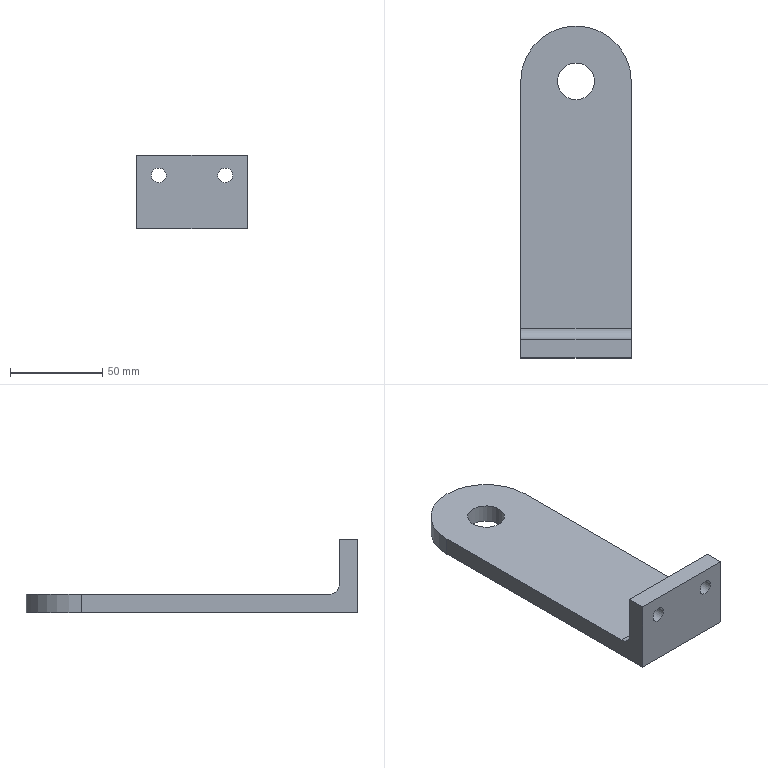Part | STEP file | tieqianzhizhu | 1 solid | 12 faces | box 60 x 180 x 40 mm | volume 118454 mm3 | plane 7 | cylinder 5 | commonest cylinder face diameters 8 x2 12 x1 20 x1 60 x1
STEP:
#1=CARTESIAN_POINT('',(0.,0.,0.));
#2=DIRECTION('',(0.,0.,1.));
#3=DIRECTION('',(1.,0.,0.));
#4=AXIS2_PLACEMENT_3D('',#1,#2,#3);
#5=CARTESIAN_POINT('',(-30.,0.,10.));
#6=VERTEX_POINT('',#5);
#7=CARTESIAN_POINT('',(-30.,-134.,10.));
#8=VERTEX_POINT('',#7);
#9=CARTESIAN_POINT('',(-30.,0.,10.));
#10=DIRECTION('',(0.,-1.,0.));
#11=VECTOR('',#10,1.);
#12=LINE('',#9,#11);
#13=CARTESIAN_POINT('',(0.,0.,10.));
#14=DIRECTION('',(0.,0.,1.));
#15=DIRECTION('',(1.,0.,0.));
#16=AXIS2_PLACEMENT_3D('',#13,#14,#15);
#17=PLANE('',#16);
#18=CARTESIAN_POINT('',(-30.,0.));
#19=DIRECTION('',(0.,-1.));
#20=VECTOR('',#19,1.);
#21=LINE('',#18,#20);
#22=(GEOMETRIC_REPRESENTATION_CONTEXT(2)PARAMETRIC_REPRESENTATION_CONTEXT()REPRESENTATION_CONTEXT('',''));
#23=DEFINITIONAL_REPRESENTATION('',(#21),#22);
#24=PCURVE('',#17,#23);
#25=CARTESIAN_POINT('',(-30.,0.,10.));
#26=DIRECTION('',(1.,0.,0.));
#27=DIRECTION('',(0.,1.,0.));
#28=AXIS2_PLACEMENT_3D('',#25,#26,#27);
#29=PLANE('',#28);
#30=CARTESIAN_POINT('',(0.,0.));
#31=DIRECTION('',(-1.,0.));
#32=VECTOR('',#31,1.);
#33=LINE('',#30,#32);
#34=(GEOMETRIC_REPRESENTATION_CONTEXT(2)PARAMETRIC_REPRESENTATION_CONTEXT()REPRESENTATION_CONTEXT('',''));
#35=DEFINITIONAL_REPRESENTATION('',(#33),#34);
#36=PCURVE('',#29,#35);
#37=SURFACE_CURVE('',#12,(#24,#36),.PCURVE_S1.);
#38=EDGE_CURVE('',#6,#8,#37,.T.);
#39=ORIENTED_EDGE('',*,*,#38,.T.);
#40=CARTESIAN_POINT('',(30.,-134.,10.));
#41=VERTEX_POINT('',#40);
#42=CARTESIAN_POINT('',(0.,-134.,10.));
#43=DIRECTION('',(1.,0.,0.));
#44=VECTOR('',#43,1.);
#45=LINE('',#42,#44);
#46=CARTESIAN_POINT('',(0.,-134.));
#47=DIRECTION('',(1.,0.));
#48=VECTOR('',#47,1.);
#49=LINE('',#46,#48);
#50=(GEOMETRIC_REPRESENTATION_CONTEXT(2)PARAMETRIC_REPRESENTATION_CONTEXT()REPRESENTATION_CONTEXT('',''));
#51=DEFINITIONAL_REPRESENTATION('',(#49),#50);
#52=PCURVE('',#17,#51);
#53=CARTESIAN_POINT('',(-30.,-134.,16.));
#54=DIRECTION('',(-1.,0.,0.));
#55=DIRECTION('',(0.,0.,1.));
#56=AXIS2_PLACEMENT_3D('',#53,#54,#55);
#57=CYLINDRICAL_SURFACE('',#56,6.);
#58=CARTESIAN_POINT('',(3.142,-30.));
#59=DIRECTION('',(0.,-1.));
#60=VECTOR('',#59,1.);
#61=LINE('',#58,#60);
#62=(GEOMETRIC_REPRESENTATION_CONTEXT(2)PARAMETRIC_REPRESENTATION_CONTEXT()REPRESENTATION_CONTEXT('',''));
#63=DEFINITIONAL_REPRESENTATION('',(#61),#62);
#64=PCURVE('',#57,#63);
#65=SURFACE_CURVE('',#45,(#52,#64),.PCURVE_S1.);
#66=EDGE_CURVE('',#8,#41,#65,.T.);
#67=ORIENTED_EDGE('',*,*,#66,.T.);
#68=CARTESIAN_POINT('',(30.,0.,10.));
#69=VERTEX_POINT('',#68);
#70=CARTESIAN_POINT('',(30.,0.,10.));
#71=DIRECTION('',(0.,1.,0.));
#72=VECTOR('',#71,1.);
#73=LINE('',#70,#72);
#74=CARTESIAN_POINT('',(30.,0.));
#75=DIRECTION('',(0.,1.));
#76=VECTOR('',#75,1.);
#77=LINE('',#74,#76);
#78=(GEOMETRIC_REPRESENTATION_CONTEXT(2)PARAMETRIC_REPRESENTATION_CONTEXT()REPRESENTATION_CONTEXT('',''));
#79=DEFINITIONAL_REPRESENTATION('',(#77),#78);
#80=PCURVE('',#17,#79);
#81=CARTESIAN_POINT('',(30.,0.,10.));
#82=DIRECTION('',(-1.,0.,0.));
#83=DIRECTION('',(0.,-1.,0.));
#84=AXIS2_PLACEMENT_3D('',#81,#82,#83);
#85=PLANE('',#84);
#86=CARTESIAN_POINT('',(0.,0.));
#87=DIRECTION('',(-1.,0.));
#88=VECTOR('',#87,1.);
#89=LINE('',#86,#88);
#90=(GEOMETRIC_REPRESENTATION_CONTEXT(2)PARAMETRIC_REPRESENTATION_CONTEXT()REPRESENTATION_CONTEXT('',''));
#91=DEFINITIONAL_REPRESENTATION('',(#89),#90);
#92=PCURVE('',#85,#91);
#93=SURFACE_CURVE('',#73,(#80,#92),.PCURVE_S1.);
#94=EDGE_CURVE('',#41,#69,#93,.T.);
#95=ORIENTED_EDGE('',*,*,#94,.T.);
#96=CARTESIAN_POINT('',(0.,0.,10.));
#97=DIRECTION('',(0.,0.,1.));
#98=DIRECTION('',(1.,0.,0.));
#99=AXIS2_PLACEMENT_3D('',#96,#97,#98);
#100=CIRCLE('',#99,30.);
#101=CARTESIAN_POINT('',(0.,0.));
#102=DIRECTION('',(1.,0.));
#103=AXIS2_PLACEMENT_2D('',#101,#102);
#104=CIRCLE('',#103,30.);
#105=(GEOMETRIC_REPRESENTATION_CONTEXT(2)PARAMETRIC_REPRESENTATION_CONTEXT()REPRESENTATION_CONTEXT('',''));
#106=DEFINITIONAL_REPRESENTATION('',(#104),#105);
#107=PCURVE('',#17,#106);
#108=CARTESIAN_POINT('',(0.,0.,10.));
#109=DIRECTION('',(0.,0.,-1.));
#110=DIRECTION('',(-1.,0.,0.));
#111=AXIS2_PLACEMENT_3D('',#108,#109,#110);
#112=CYLINDRICAL_SURFACE('',#111,30.);
#113=CARTESIAN_POINT('',(3.142,0.));
#114=DIRECTION('',(-1.,0.));
#115=VECTOR('',#114,1.);
#116=LINE('',#113,#115);
#117=(GEOMETRIC_REPRESENTATION_CONTEXT(2)PARAMETRIC_REPRESENTATION_CONTEXT()REPRESENTATION_CONTEXT('',''));
#118=DEFINITIONAL_REPRESENTATION('',(#116),#117);
#119=PCURVE('',#112,#118);
#120=SURFACE_CURVE('',#100,(#107,#119),.PCURVE_S1.);
#121=EDGE_CURVE('',#69,#6,#120,.T.);
#122=ORIENTED_EDGE('',*,*,#121,.T.);
#123=EDGE_LOOP('',(#39,#67,#95,#122));
#124=FACE_BOUND('',#123,.T.);
#125=CARTESIAN_POINT('',(10.,0.,10.));
#126=VERTEX_POINT('',#125);
#127=CARTESIAN_POINT('',(0.,0.,10.));
#128=DIRECTION('',(0.,0.,1.));
#129=DIRECTION('',(1.,0.,0.));
#130=AXIS2_PLACEMENT_3D('',#127,#128,#129);
#131=CIRCLE('',#130,10.);
#132=CARTESIAN_POINT('',(0.,0.));
#133=DIRECTION('',(1.,0.));
#134=AXIS2_PLACEMENT_2D('',#132,#133);
#135=CIRCLE('',#134,10.);
#136=(GEOMETRIC_REPRESENTATION_CONTEXT(2)PARAMETRIC_REPRESENTATION_CONTEXT()REPRESENTATION_CONTEXT('',''));
#137=DEFINITIONAL_REPRESENTATION('',(#135),#136);
#138=PCURVE('',#17,#137);
#139=CARTESIAN_POINT('',(0.,0.,10.));
#140=DIRECTION('',(0.,0.,-1.));
#141=DIRECTION('',(-1.,0.,0.));
#142=AXIS2_PLACEMENT_3D('',#139,#140,#141);
#143=CYLINDRICAL_SURFACE('',#142,10.);
#144=CARTESIAN_POINT('',(9.425,0.));
#145=DIRECTION('',(-1.,0.));
#146=VECTOR('',#145,1.);
#147=LINE('',#144,#146);
#148=(GEOMETRIC_REPRESENTATION_CONTEXT(2)PARAMETRIC_REPRESENTATION_CONTEXT()REPRESENTATION_CONTEXT('',''));
#149=DEFINITIONAL_REPRESENTATION('',(#147),#148);
#150=PCURVE('',#143,#149);
#151=SURFACE_CURVE('',#131,(#138,#150),.PCURVE_S1.);
#152=EDGE_CURVE('',#126,#126,#151,.T.);
#153=ORIENTED_EDGE('',*,*,#152,.F.);
#154=EDGE_LOOP('',(#153));
#155=FACE_BOUND('',#154,.T.);
#156=ADVANCED_FACE('',(#124,#155),#17,.T.);
#157=CARTESIAN_POINT('',(30.,0.,0.));
#158=VERTEX_POINT('',#157);
#159=CARTESIAN_POINT('',(-30.,0.,0.));
#160=VERTEX_POINT('',#159);
#161=CARTESIAN_POINT('',(0.,0.,0.));
#162=DIRECTION('',(0.,0.,1.));
#163=DIRECTION('',(1.,0.,0.));
#164=AXIS2_PLACEMENT_3D('',#161,#162,#163);
#165=CIRCLE('',#164,30.);
#166=CARTESIAN_POINT('',(0.,0.,0.));
#167=DIRECTION('',(0.,0.,1.));
#168=DIRECTION('',(1.,0.,0.));
#169=AXIS2_PLACEMENT_3D('',#166,#167,#168);
#170=PLANE('',#169);
#171=CARTESIAN_POINT('',(0.,0.));
#172=DIRECTION('',(1.,0.));
#173=AXIS2_PLACEMENT_2D('',#171,#172);
#174=CIRCLE('',#173,30.);
#175=(GEOMETRIC_REPRESENTATION_CONTEXT(2)PARAMETRIC_REPRESENTATION_CONTEXT()REPRESENTATION_CONTEXT('',''));
#176=DEFINITIONAL_REPRESENTATION('',(#174),#175);
#177=PCURVE('',#170,#176);
#178=CARTESIAN_POINT('',(3.142,10.));
#179=DIRECTION('',(-1.,0.));
#180=VECTOR('',#179,1.);
#181=LINE('',#178,#180);
#182=(GEOMETRIC_REPRESENTATION_CONTEXT(2)PARAMETRIC_REPRESENTATION_CONTEXT()REPRESENTATION_CONTEXT('',''));
#183=DEFINITIONAL_REPRESENTATION('',(#181),#182);
#184=PCURVE('',#112,#183);
#185=SURFACE_CURVE('',#165,(#177,#184),.PCURVE_S1.);
#186=EDGE_CURVE('',#158,#160,#185,.T.);
#187=ORIENTED_EDGE('',*,*,#186,.F.);
#188=CARTESIAN_POINT('',(30.,-150.,0.));
#189=VERTEX_POINT('',#188);
#190=CARTESIAN_POINT('',(30.,0.,0.));
#191=DIRECTION('',(0.,1.,0.));
#192=VECTOR('',#191,1.);
#193=LINE('',#190,#192);
#194=CARTESIAN_POINT('',(30.,0.));
#195=DIRECTION('',(0.,1.));
#196=VECTOR('',#195,1.);
#197=LINE('',#194,#196);
#198=(GEOMETRIC_REPRESENTATION_CONTEXT(2)PARAMETRIC_REPRESENTATION_CONTEXT()REPRESENTATION_CONTEXT('',''));
#199=DEFINITIONAL_REPRESENTATION('',(#197),#198);
#200=PCURVE('',#170,#199);
#201=CARTESIAN_POINT('',(0.,-10.));
#202=DIRECTION('',(-1.,0.));
#203=VECTOR('',#202,1.);
#204=LINE('',#201,#203);
#205=(GEOMETRIC_REPRESENTATION_CONTEXT(2)PARAMETRIC_REPRESENTATION_CONTEXT()REPRESENTATION_CONTEXT('',''));
#206=DEFINITIONAL_REPRESENTATION('',(#204),#205);
#207=PCURVE('',#85,#206);
#208=SURFACE_CURVE('',#193,(#200,#207),.PCURVE_S1.);
#209=EDGE_CURVE('',#189,#158,#208,.T.);
#210=ORIENTED_EDGE('',*,*,#209,.F.);
#211=CARTESIAN_POINT('',(-30.,-150.,0.));
#212=VERTEX_POINT('',#211);
#213=CARTESIAN_POINT('',(30.,-150.,0.));
#214=DIRECTION('',(1.,0.,0.));
#215=VECTOR('',#214,1.);
#216=LINE('',#213,#215);
#217=CARTESIAN_POINT('',(30.,-150.));
#218=DIRECTION('',(1.,0.));
#219=VECTOR('',#218,1.);
#220=LINE('',#217,#219);
#221=(GEOMETRIC_REPRESENTATION_CONTEXT(2)PARAMETRIC_REPRESENTATION_CONTEXT()REPRESENTATION_CONTEXT('',''));
#222=DEFINITIONAL_REPRESENTATION('',(#220),#221);
#223=PCURVE('',#170,#222);
#224=CARTESIAN_POINT('',(30.,-150.,10.));
#225=DIRECTION('',(0.,1.,0.));
#226=DIRECTION('',(-1.,0.,0.));
#227=AXIS2_PLACEMENT_3D('',#224,#225,#226);
#228=PLANE('',#227);
#229=CARTESIAN_POINT('',(0.,-10.));
#230=DIRECTION('',(-1.,0.));
#231=VECTOR('',#230,1.);
#232=LINE('',#229,#231);
#233=(GEOMETRIC_REPRESENTATION_CONTEXT(2)PARAMETRIC_REPRESENTATION_CONTEXT()REPRESENTATION_CONTEXT('',''));
#234=DEFINITIONAL_REPRESENTATION('',(#232),#233);
#235=PCURVE('',#228,#234);
#236=SURFACE_CURVE('',#216,(#223,#235),.PCURVE_S1.);
#237=EDGE_CURVE('',#212,#189,#236,.T.);
#238=ORIENTED_EDGE('',*,*,#237,.F.);
#239=CARTESIAN_POINT('',(-30.,0.,0.));
#240=DIRECTION('',(0.,-1.,0.));
#241=VECTOR('',#240,1.);
#242=LINE('',#239,#241);
#243=CARTESIAN_POINT('',(-30.,0.));
#244=DIRECTION('',(0.,-1.));
#245=VECTOR('',#244,1.);
#246=LINE('',#243,#245);
#247=(GEOMETRIC_REPRESENTATION_CONTEXT(2)PARAMETRIC_REPRESENTATION_CONTEXT()REPRESENTATION_CONTEXT('',''));
#248=DEFINITIONAL_REPRESENTATION('',(#246),#247);
#249=PCURVE('',#170,#248);
#250=CARTESIAN_POINT('',(0.,-10.));
#251=DIRECTION('',(-1.,0.));
#252=VECTOR('',#251,1.);
#253=LINE('',#250,#252);
#254=(GEOMETRIC_REPRESENTATION_CONTEXT(2)PARAMETRIC_REPRESENTATION_CONTEXT()REPRESENTATION_CONTEXT('',''));
#255=DEFINITIONAL_REPRESENTATION('',(#253),#254);
#256=PCURVE('',#29,#255);
#257=SURFACE_CURVE('',#242,(#249,#256),.PCURVE_S1.);
#258=EDGE_CURVE('',#160,#212,#257,.T.);
#259=ORIENTED_EDGE('',*,*,#258,.F.);
#260=EDGE_LOOP('',(#187,#210,#238,#259));
#261=FACE_BOUND('',#260,.T.);
#262=CARTESIAN_POINT('',(10.,0.,0.));
#263=VERTEX_POINT('',#262);
#264=CARTESIAN_POINT('',(0.,0.,0.));
#265=DIRECTION('',(0.,0.,1.));
#266=DIRECTION('',(1.,0.,0.));
#267=AXIS2_PLACEMENT_3D('',#264,#265,#266);
#268=CIRCLE('',#267,10.);
#269=CARTESIAN_POINT('',(0.,0.));
#270=DIRECTION('',(1.,0.));
#271=AXIS2_PLACEMENT_2D('',#269,#270);
#272=CIRCLE('',#271,10.);
#273=(GEOMETRIC_REPRESENTATION_CONTEXT(2)PARAMETRIC_REPRESENTATION_CONTEXT()REPRESENTATION_CONTEXT('',''));
#274=DEFINITIONAL_REPRESENTATION('',(#272),#273);
#275=PCURVE('',#170,#274);
#276=CARTESIAN_POINT('',(9.425,10.));
#277=DIRECTION('',(-1.,0.));
#278=VECTOR('',#277,1.);
#279=LINE('',#276,#278);
#280=(GEOMETRIC_REPRESENTATION_CONTEXT(2)PARAMETRIC_REPRESENTATION_CONTEXT()REPRESENTATION_CONTEXT('',''));
#281=DEFINITIONAL_REPRESENTATION('',(#279),#280);
#282=PCURVE('',#143,#281);
#283=SURFACE_CURVE('',#268,(#275,#282),.PCURVE_S1.);
#284=EDGE_CURVE('',#263,#263,#283,.T.);
#285=ORIENTED_EDGE('',*,*,#284,.T.);
#286=EDGE_LOOP('',(#285));
#287=FACE_BOUND('',#286,.T.);
#288=ADVANCED_FACE('',(#261,#287),#170,.F.);
#289=ORIENTED_EDGE('',*,*,#186,.T.);
#290=CARTESIAN_POINT('',(-30.,0.,10.));
#291=DIRECTION('',(0.,0.,-1.));
#292=VECTOR('',#291,1.);
#293=LINE('',#290,#292);
#294=CARTESIAN_POINT('',(0.,0.));
#295=DIRECTION('',(0.,1.));
#296=VECTOR('',#295,1.);
#297=LINE('',#294,#296);
#298=(GEOMETRIC_REPRESENTATION_CONTEXT(2)PARAMETRIC_REPRESENTATION_CONTEXT()REPRESENTATION_CONTEXT('',''));
#299=DEFINITIONAL_REPRESENTATION('',(#297),#298);
#300=PCURVE('',#112,#299);
#301=CARTESIAN_POINT('',(0.,0.));
#302=DIRECTION('',(0.,-1.));
#303=VECTOR('',#302,1.);
#304=LINE('',#301,#303);
#305=(GEOMETRIC_REPRESENTATION_CONTEXT(2)PARAMETRIC_REPRESENTATION_CONTEXT()REPRESENTATION_CONTEXT('',''));
#306=DEFINITIONAL_REPRESENTATION('',(#304),#305);
#307=PCURVE('',#29,#306);
#308=SURFACE_CURVE('',#293,(#300,#307),.PCURVE_S1.);
#309=EDGE_CURVE('',#6,#160,#308,.T.);
#310=ORIENTED_EDGE('',*,*,#309,.F.);
#311=ORIENTED_EDGE('',*,*,#121,.F.);
#312=CARTESIAN_POINT('',(30.,0.,10.));
#313=DIRECTION('',(0.,0.,-1.));
#314=VECTOR('',#313,1.);
#315=LINE('',#312,#314);
#316=CARTESIAN_POINT('',(3.142,0.));
#317=DIRECTION('',(0.,1.));
#318=VECTOR('',#317,1.);
#319=LINE('',#316,#318);
#320=(GEOMETRIC_REPRESENTATION_CONTEXT(2)PARAMETRIC_REPRESENTATION_CONTEXT()REPRESENTATION_CONTEXT('',''));
#321=DEFINITIONAL_REPRESENTATION('',(#319),#320);
#322=PCURVE('',#112,#321);
#323=CARTESIAN_POINT('',(0.,0.));
#324=DIRECTION('',(0.,-1.));
#325=VECTOR('',#324,1.);
#326=LINE('',#323,#325);
#327=(GEOMETRIC_REPRESENTATION_CONTEXT(2)PARAMETRIC_REPRESENTATION_CONTEXT()REPRESENTATION_CONTEXT('',''));
#328=DEFINITIONAL_REPRESENTATION('',(#326),#327);
#329=PCURVE('',#85,#328);
#330=SURFACE_CURVE('',#315,(#322,#329),.PCURVE_S1.);
#331=EDGE_CURVE('',#69,#158,#330,.T.);
#332=ORIENTED_EDGE('',*,*,#331,.T.);
#333=EDGE_LOOP('',(#289,#310,#311,#332));
#334=FACE_BOUND('',#333,.T.);
#335=ADVANCED_FACE('',(#334),#112,.T.);
#336=ORIENTED_EDGE('',*,*,#258,.T.);
#337=CARTESIAN_POINT('',(-30.,-150.,40.));
#338=VERTEX_POINT('',#337);
#339=CARTESIAN_POINT('',(-30.,-150.,10.));
#340=DIRECTION('',(0.,0.,-1.));
#341=VECTOR('',#340,1.);
#342=LINE('',#339,#341);
#343=CARTESIAN_POINT('',(-150.,0.));
#344=DIRECTION('',(0.,-1.));
#345=VECTOR('',#344,1.);
#346=LINE('',#343,#345);
#347=(GEOMETRIC_REPRESENTATION_CONTEXT(2)PARAMETRIC_REPRESENTATION_CONTEXT()REPRESENTATION_CONTEXT('',''));
#348=DEFINITIONAL_REPRESENTATION('',(#346),#347);
#349=PCURVE('',#29,#348);
#350=CARTESIAN_POINT('',(60.,0.));
#351=DIRECTION('',(0.,-1.));
#352=VECTOR('',#351,1.);
#353=LINE('',#350,#352);
#354=(GEOMETRIC_REPRESENTATION_CONTEXT(2)PARAMETRIC_REPRESENTATION_CONTEXT()REPRESENTATION_CONTEXT('',''));
#355=DEFINITIONAL_REPRESENTATION('',(#353),#354);
#356=PCURVE('',#228,#355);
#357=SURFACE_CURVE('',#342,(#349,#356),.PCURVE_S1.);
#358=EDGE_CURVE('',#338,#212,#357,.T.);
#359=ORIENTED_EDGE('',*,*,#358,.F.);
#360=CARTESIAN_POINT('',(-30.,-140.,40.));
#361=VERTEX_POINT('',#360);
#362=CARTESIAN_POINT('',(-30.,-150.,40.));
#363=DIRECTION('',(0.,-1.,0.));
#364=VECTOR('',#363,1.);
#365=LINE('',#362,#364);
#366=CARTESIAN_POINT('',(-150.,30.));
#367=DIRECTION('',(-1.,0.));
#368=VECTOR('',#367,1.);
#369=LINE('',#366,#368);
#370=(GEOMETRIC_REPRESENTATION_CONTEXT(2)PARAMETRIC_REPRESENTATION_CONTEXT()REPRESENTATION_CONTEXT('',''));
#371=DEFINITIONAL_REPRESENTATION('',(#369),#370);
#372=PCURVE('',#29,#371);
#373=CARTESIAN_POINT('',(0.,0.,40.));
#374=DIRECTION('',(0.,0.,-1.));
#375=DIRECTION('',(-1.,0.,0.));
#376=AXIS2_PLACEMENT_3D('',#373,#374,#375);
#377=PLANE('',#376);
#378=CARTESIAN_POINT('',(30.,-150.));
#379=DIRECTION('',(0.,-1.));
#380=VECTOR('',#379,1.);
#381=LINE('',#378,#380);
#382=(GEOMETRIC_REPRESENTATION_CONTEXT(2)PARAMETRIC_REPRESENTATION_CONTEXT()REPRESENTATION_CONTEXT('',''));
#383=DEFINITIONAL_REPRESENTATION('',(#381),#382);
#384=PCURVE('',#377,#383);
#385=SURFACE_CURVE('',#365,(#372,#384),.PCURVE_S1.);
#386=EDGE_CURVE('',#361,#338,#385,.T.);
#387=ORIENTED_EDGE('',*,*,#386,.F.);
#388=CARTESIAN_POINT('',(-30.,-140.,16.));
#389=VERTEX_POINT('',#388);
#390=CARTESIAN_POINT('',(-30.,-140.,40.));
#391=DIRECTION('',(0.,0.,-1.));
#392=VECTOR('',#391,1.);
#393=LINE('',#390,#392);
#394=CARTESIAN_POINT('',(-140.,30.));
#395=DIRECTION('',(0.,-1.));
#396=VECTOR('',#395,1.);
#397=LINE('',#394,#396);
#398=(GEOMETRIC_REPRESENTATION_CONTEXT(2)PARAMETRIC_REPRESENTATION_CONTEXT()REPRESENTATION_CONTEXT('',''));
#399=DEFINITIONAL_REPRESENTATION('',(#397),#398);
#400=PCURVE('',#29,#399);
#401=CARTESIAN_POINT('',(-30.,-140.,40.));
#402=DIRECTION('',(0.,-1.,0.));
#403=DIRECTION('',(0.,0.,-1.));
#404=AXIS2_PLACEMENT_3D('',#401,#402,#403);
#405=PLANE('',#404);
#406=CARTESIAN_POINT('',(0.,0.));
#407=DIRECTION('',(1.,0.));
#408=VECTOR('',#407,1.);
#409=LINE('',#406,#408);
#410=(GEOMETRIC_REPRESENTATION_CONTEXT(2)PARAMETRIC_REPRESENTATION_CONTEXT()REPRESENTATION_CONTEXT('',''));
#411=DEFINITIONAL_REPRESENTATION('',(#409),#410);
#412=PCURVE('',#405,#411);
#413=SURFACE_CURVE('',#393,(#400,#412),.PCURVE_S1.);
#414=EDGE_CURVE('',#361,#389,#413,.T.);
#415=ORIENTED_EDGE('',*,*,#414,.T.);
#416=CARTESIAN_POINT('',(-30.,-134.,16.));
#417=DIRECTION('',(1.,0.,0.));
#418=DIRECTION('',(0.,1.,0.));
#419=AXIS2_PLACEMENT_3D('',#416,#417,#418);
#420=CIRCLE('',#419,6.);
#421=CARTESIAN_POINT('',(-134.,6.));
#422=DIRECTION('',(1.,0.));
#423=AXIS2_PLACEMENT_2D('',#421,#422);
#424=CIRCLE('',#423,6.);
#425=(GEOMETRIC_REPRESENTATION_CONTEXT(2)PARAMETRIC_REPRESENTATION_CONTEXT()REPRESENTATION_CONTEXT('',''));
#426=DEFINITIONAL_REPRESENTATION('',(#424),#425);
#427=PCURVE('',#29,#426);
#428=CARTESIAN_POINT('',(7.854,0.));
#429=DIRECTION('',(-1.,0.));
#430=VECTOR('',#429,1.);
#431=LINE('',#428,#430);
#432=(GEOMETRIC_REPRESENTATION_CONTEXT(2)PARAMETRIC_REPRESENTATION_CONTEXT()REPRESENTATION_CONTEXT('',''));
#433=DEFINITIONAL_REPRESENTATION('',(#431),#432);
#434=PCURVE('',#57,#433);
#435=SURFACE_CURVE('',#420,(#427,#434),.PCURVE_S1.);
#436=EDGE_CURVE('',#389,#8,#435,.T.);
#437=ORIENTED_EDGE('',*,*,#436,.T.);
#438=ORIENTED_EDGE('',*,*,#38,.F.);
#439=ORIENTED_EDGE('',*,*,#309,.T.);
#440=EDGE_LOOP('',(#336,#359,#387,#415,#437,#438,#439));
#441=FACE_BOUND('',#440,.T.);
#442=ADVANCED_FACE('',(#441),#29,.F.);
#443=CARTESIAN_POINT('',(18.,-150.,33.));
#444=VERTEX_POINT('',#443);
#445=CARTESIAN_POINT('',(18.,-150.,29.));
#446=DIRECTION('',(0.,1.,0.));
#447=DIRECTION('',(0.,0.,1.));
#448=AXIS2_PLACEMENT_3D('',#445,#446,#447);
#449=CIRCLE('',#448,4.);
#450=CARTESIAN_POINT('',(12.,19.));
#451=DIRECTION('',(0.,1.));
#452=AXIS2_PLACEMENT_2D('',#450,#451);
#453=CIRCLE('',#452,4.);
#454=(GEOMETRIC_REPRESENTATION_CONTEXT(2)PARAMETRIC_REPRESENTATION_CONTEXT()REPRESENTATION_CONTEXT('',''));
#455=DEFINITIONAL_REPRESENTATION('',(#453),#454);
#456=PCURVE('',#228,#455);
#457=CARTESIAN_POINT('',(18.,-150.,29.));
#458=DIRECTION('',(0.,1.,0.));
#459=DIRECTION('',(0.,0.,1.));
#460=AXIS2_PLACEMENT_3D('',#457,#458,#459);
#461=CYLINDRICAL_SURFACE('',#460,4.);
#462=CARTESIAN_POINT('',(0.,0.));
#463=DIRECTION('',(1.,0.));
#464=VECTOR('',#463,1.);
#465=LINE('',#462,#464);
#466=(GEOMETRIC_REPRESENTATION_CONTEXT(2)PARAMETRIC_REPRESENTATION_CONTEXT()REPRESENTATION_CONTEXT('',''));
#467=DEFINITIONAL_REPRESENTATION('',(#465),#466);
#468=PCURVE('',#461,#467);
#469=SURFACE_CURVE('',#449,(#456,#468),.PCURVE_S1.);
#470=EDGE_CURVE('',#444,#444,#469,.T.);
#471=ORIENTED_EDGE('',*,*,#470,.T.);
#472=EDGE_LOOP('',(#471));
#473=FACE_BOUND('',#472,.T.);
#474=CARTESIAN_POINT('',(-18.,-150.,33.));
#475=VERTEX_POINT('',#474);
#476=CARTESIAN_POINT('',(-18.,-150.,29.));
#477=DIRECTION('',(0.,1.,0.));
#478=DIRECTION('',(0.,0.,1.));
#479=AXIS2_PLACEMENT_3D('',#476,#477,#478);
#480=CIRCLE('',#479,4.);
#481=CARTESIAN_POINT('',(48.,19.));
#482=DIRECTION('',(0.,1.));
#483=AXIS2_PLACEMENT_2D('',#481,#482);
#484=CIRCLE('',#483,4.);
#485=(GEOMETRIC_REPRESENTATION_CONTEXT(2)PARAMETRIC_REPRESENTATION_CONTEXT()REPRESENTATION_CONTEXT('',''));
#486=DEFINITIONAL_REPRESENTATION('',(#484),#485);
#487=PCURVE('',#228,#486);
#488=CARTESIAN_POINT('',(-18.,-150.,29.));
#489=DIRECTION('',(0.,1.,0.));
#490=DIRECTION('',(0.,0.,1.));
#491=AXIS2_PLACEMENT_3D('',#488,#489,#490);
#492=CYLINDRICAL_SURFACE('',#491,4.);
#493=CARTESIAN_POINT('',(0.,0.));
#494=DIRECTION('',(1.,0.));
#495=VECTOR('',#494,1.);
#496=LINE('',#493,#495);
#497=(GEOMETRIC_REPRESENTATION_CONTEXT(2)PARAMETRIC_REPRESENTATION_CONTEXT()REPRESENTATION_CONTEXT('',''));
#498=DEFINITIONAL_REPRESENTATION('',(#496),#497);
#499=PCURVE('',#492,#498);
#500=SURFACE_CURVE('',#480,(#487,#499),.PCURVE_S1.);
#501=EDGE_CURVE('',#475,#475,#500,.T.);
#502=ORIENTED_EDGE('',*,*,#501,.T.);
#503=EDGE_LOOP('',(#502));
#504=FACE_BOUND('',#503,.T.);
#505=ORIENTED_EDGE('',*,*,#237,.T.);
#506=CARTESIAN_POINT('',(30.,-150.,40.));
#507=VERTEX_POINT('',#506);
#508=CARTESIAN_POINT('',(30.,-150.,10.));
#509=DIRECTION('',(0.,0.,-1.));
#510=VECTOR('',#509,1.);
#511=LINE('',#508,#510);
#512=CARTESIAN_POINT('',(0.,0.));
#513=DIRECTION('',(0.,-1.));
#514=VECTOR('',#513,1.);
#515=LINE('',#512,#514);
#516=(GEOMETRIC_REPRESENTATION_CONTEXT(2)PARAMETRIC_REPRESENTATION_CONTEXT()REPRESENTATION_CONTEXT('',''));
#517=DEFINITIONAL_REPRESENTATION('',(#515),#516);
#518=PCURVE('',#228,#517);
#519=CARTESIAN_POINT('',(150.,0.));
#520=DIRECTION('',(0.,-1.));
#521=VECTOR('',#520,1.);
#522=LINE('',#519,#521);
#523=(GEOMETRIC_REPRESENTATION_CONTEXT(2)PARAMETRIC_REPRESENTATION_CONTEXT()REPRESENTATION_CONTEXT('',''));
#524=DEFINITIONAL_REPRESENTATION('',(#522),#523);
#525=PCURVE('',#85,#524);
#526=SURFACE_CURVE('',#511,(#518,#525),.PCURVE_S1.);
#527=EDGE_CURVE('',#507,#189,#526,.T.);
#528=ORIENTED_EDGE('',*,*,#527,.F.);
#529=CARTESIAN_POINT('',(-30.,-150.,40.));
#530=DIRECTION('',(1.,0.,0.));
#531=VECTOR('',#530,1.);
#532=LINE('',#529,#531);
#533=CARTESIAN_POINT('',(60.,30.));
#534=DIRECTION('',(-1.,0.));
#535=VECTOR('',#534,1.);
#536=LINE('',#533,#535);
#537=(GEOMETRIC_REPRESENTATION_CONTEXT(2)PARAMETRIC_REPRESENTATION_CONTEXT()REPRESENTATION_CONTEXT('',''));
#538=DEFINITIONAL_REPRESENTATION('',(#536),#537);
#539=PCURVE('',#228,#538);
#540=CARTESIAN_POINT('',(30.,-150.));
#541=DIRECTION('',(-1.,0.));
#542=VECTOR('',#541,1.);
#543=LINE('',#540,#542);
#544=(GEOMETRIC_REPRESENTATION_CONTEXT(2)PARAMETRIC_REPRESENTATION_CONTEXT()REPRESENTATION_CONTEXT('',''));
#545=DEFINITIONAL_REPRESENTATION('',(#543),#544);
#546=PCURVE('',#377,#545);
#547=SURFACE_CURVE('',#532,(#539,#546),.PCURVE_S1.);
#548=EDGE_CURVE('',#338,#507,#547,.T.);
#549=ORIENTED_EDGE('',*,*,#548,.F.);
#550=ORIENTED_EDGE('',*,*,#358,.T.);
#551=EDGE_LOOP('',(#505,#528,#549,#550));
#552=FACE_BOUND('',#551,.T.);
#553=ADVANCED_FACE('',(#473,#504,#552),#228,.F.);
#554=ORIENTED_EDGE('',*,*,#209,.T.);
#555=ORIENTED_EDGE('',*,*,#331,.F.);
#556=ORIENTED_EDGE('',*,*,#94,.F.);
#557=CARTESIAN_POINT('',(30.,-140.,16.));
#558=VERTEX_POINT('',#557);
#559=CARTESIAN_POINT('',(30.,-134.,16.));
#560=DIRECTION('',(-1.,0.,0.));
#561=DIRECTION('',(0.,-1.,0.));
#562=AXIS2_PLACEMENT_3D('',#559,#560,#561);
#563=CIRCLE('',#562,6.);
#564=CARTESIAN_POINT('',(134.,6.));
#565=DIRECTION('',(1.,0.));
#566=AXIS2_PLACEMENT_2D('',#564,#565);
#567=CIRCLE('',#566,6.);
#568=(GEOMETRIC_REPRESENTATION_CONTEXT(2)PARAMETRIC_REPRESENTATION_CONTEXT()REPRESENTATION_CONTEXT('',''));
#569=DEFINITIONAL_REPRESENTATION('',(#567),#568);
#570=PCURVE('',#85,#569);
#571=CARTESIAN_POINT('',(-1.571,-60.));
#572=DIRECTION('',(1.,0.));
#573=VECTOR('',#572,1.);
#574=LINE('',#571,#573);
#575=(GEOMETRIC_REPRESENTATION_CONTEXT(2)PARAMETRIC_REPRESENTATION_CONTEXT()REPRESENTATION_CONTEXT('',''));
#576=DEFINITIONAL_REPRESENTATION('',(#574),#575);
#577=PCURVE('',#57,#576);
#578=SURFACE_CURVE('',#563,(#570,#577),.PCURVE_S1.);
#579=EDGE_CURVE('',#41,#558,#578,.T.);
#580=ORIENTED_EDGE('',*,*,#579,.T.);
#581=CARTESIAN_POINT('',(30.,-140.,40.));
#582=VERTEX_POINT('',#581);
#583=CARTESIAN_POINT('',(30.,-140.,40.));
#584=DIRECTION('',(0.,0.,-1.));
#585=VECTOR('',#584,1.);
#586=LINE('',#583,#585);
#587=CARTESIAN_POINT('',(140.,30.));
#588=DIRECTION('',(0.,-1.));
#589=VECTOR('',#588,1.);
#590=LINE('',#587,#589);
#591=(GEOMETRIC_REPRESENTATION_CONTEXT(2)PARAMETRIC_REPRESENTATION_CONTEXT()REPRESENTATION_CONTEXT('',''));
#592=DEFINITIONAL_REPRESENTATION('',(#590),#591);
#593=PCURVE('',#85,#592);
#594=CARTESIAN_POINT('',(0.,60.));
#595=DIRECTION('',(1.,0.));
#596=VECTOR('',#595,1.);
#597=LINE('',#594,#596);
#598=(GEOMETRIC_REPRESENTATION_CONTEXT(2)PARAMETRIC_REPRESENTATION_CONTEXT()REPRESENTATION_CONTEXT('',''));
#599=DEFINITIONAL_REPRESENTATION('',(#597),#598);
#600=PCURVE('',#405,#599);
#601=SURFACE_CURVE('',#586,(#593,#600),.PCURVE_S1.);
#602=EDGE_CURVE('',#582,#558,#601,.T.);
#603=ORIENTED_EDGE('',*,*,#602,.F.);
#604=CARTESIAN_POINT('',(30.,-150.,40.));
#605=DIRECTION('',(0.,1.,0.));
#606=VECTOR('',#605,1.);
#607=LINE('',#604,#606);
#608=CARTESIAN_POINT('',(150.,30.));
#609=DIRECTION('',(-1.,0.));
#610=VECTOR('',#609,1.);
#611=LINE('',#608,#610);
#612=(GEOMETRIC_REPRESENTATION_CONTEXT(2)PARAMETRIC_REPRESENTATION_CONTEXT()REPRESENTATION_CONTEXT('',''));
#613=DEFINITIONAL_REPRESENTATION('',(#611),#612);
#614=PCURVE('',#85,#613);
#615=CARTESIAN_POINT('',(-30.,-150.));
#616=DIRECTION('',(0.,1.));
#617=VECTOR('',#616,1.);
#618=LINE('',#615,#617);
#619=(GEOMETRIC_REPRESENTATION_CONTEXT(2)PARAMETRIC_REPRESENTATION_CONTEXT()REPRESENTATION_CONTEXT('',''));
#620=DEFINITIONAL_REPRESENTATION('',(#618),#619);
#621=PCURVE('',#377,#620);
#622=SURFACE_CURVE('',#607,(#614,#621),.PCURVE_S1.);
#623=EDGE_CURVE('',#507,#582,#622,.T.);
#624=ORIENTED_EDGE('',*,*,#623,.F.);
#625=ORIENTED_EDGE('',*,*,#527,.T.);
#626=EDGE_LOOP('',(#554,#555,#556,#580,#603,#624,#625));
#627=FACE_BOUND('',#626,.T.);
#628=ADVANCED_FACE('',(#627),#85,.F.);
#629=ORIENTED_EDGE('',*,*,#152,.F.);
#630=CARTESIAN_POINT('',(10.,0.,10.));
#631=CARTESIAN_POINT('',(10.,0.,0.));
#632=B_SPLINE_CURVE_WITH_KNOTS('',1,(#630,#631),.UNSPECIFIED.,.F.,.F.,(2,2),(0.,10.),.PIECEWISE_BEZIER_KNOTS.);
#633=CARTESIAN_POINT('',(9.425,0.));
#634=DIRECTION('',(0.,1.));
#635=VECTOR('',#634,1.);
#636=LINE('',#633,#635);
#637=(GEOMETRIC_REPRESENTATION_CONTEXT(2)PARAMETRIC_REPRESENTATION_CONTEXT()REPRESENTATION_CONTEXT('',''));
#638=DEFINITIONAL_REPRESENTATION('',(#636),#637);
#639=PCURVE('',#143,#638);
#640=CARTESIAN_POINT('',(3.142,0.));
#641=DIRECTION('',(0.,1.));
#642=VECTOR('',#641,1.);
#643=LINE('',#640,#642);
#644=(GEOMETRIC_REPRESENTATION_CONTEXT(2)PARAMETRIC_REPRESENTATION_CONTEXT()REPRESENTATION_CONTEXT('',''));
#645=DEFINITIONAL_REPRESENTATION('',(#643),#644);
#646=PCURVE('',#143,#645);
#647=SEAM_CURVE('',#632,(#639,#646),.PCURVE_S1.);
#648=EDGE_CURVE('',#126,#263,#647,.T.);
#649=ORIENTED_EDGE('',*,*,#648,.T.);
#650=ORIENTED_EDGE('',*,*,#284,.T.);
#651=ORIENTED_EDGE('',*,*,#648,.F.);
#652=EDGE_LOOP('',(#629,#649,#650,#651));
#653=FACE_BOUND('',#652,.F.);
#654=ADVANCED_FACE('',(#653),#143,.F.);
#655=CARTESIAN_POINT('',(18.,-140.,33.));
#656=VERTEX_POINT('',#655);
#657=CARTESIAN_POINT('',(18.,-140.,29.));
#658=DIRECTION('',(0.,1.,0.));
#659=DIRECTION('',(0.,0.,1.));
#660=AXIS2_PLACEMENT_3D('',#657,#658,#659);
#661=CIRCLE('',#660,4.);
#662=CARTESIAN_POINT('',(7.,48.));
#663=CARTESIAN_POINT('',(7.,54.928));
#664=CARTESIAN_POINT('',(13.,51.464));
#665=CARTESIAN_POINT('',(19.,48.));
#666=CARTESIAN_POINT('',(13.,44.536));
#667=CARTESIAN_POINT('',(7.,41.072));
#668=CARTESIAN_POINT('',(7.,48.));
#669=(BOUNDED_CURVE()B_SPLINE_CURVE(2,(#662,#663,#664,#665,#666,#667,#668),.UNSPECIFIED.,.T.,.F.)B_SPLINE_CURVE_WITH_KNOTS((1,2,2,2,2,1),(-2.094,0.,2.094,4.189,6.283,8.378),.UNSPECIFIED.)CURVE()GEOMETRIC_REPRESENTATION_ITEM()RATIONAL_B_SPLINE_CURVE((1.,0.5,1.,0.5,1.,0.5,1.))REPRESENTATION_ITEM(''));
#670=(GEOMETRIC_REPRESENTATION_CONTEXT(2)PARAMETRIC_REPRESENTATION_CONTEXT()REPRESENTATION_CONTEXT('',''));
#671=DEFINITIONAL_REPRESENTATION('',(#669),#670);
#672=PCURVE('',#405,#671);
#673=CARTESIAN_POINT('',(0.,10.));
#674=DIRECTION('',(1.,0.));
#675=VECTOR('',#674,1.);
#676=LINE('',#673,#675);
#677=(GEOMETRIC_REPRESENTATION_CONTEXT(2)PARAMETRIC_REPRESENTATION_CONTEXT()REPRESENTATION_CONTEXT('',''));
#678=DEFINITIONAL_REPRESENTATION('',(#676),#677);
#679=PCURVE('',#461,#678);
#680=SURFACE_CURVE('',#661,(#672,#679),.PCURVE_S1.);
#681=EDGE_CURVE('',#656,#656,#680,.T.);
#682=ORIENTED_EDGE('',*,*,#681,.F.);
#683=EDGE_LOOP('',(#682));
#684=FACE_BOUND('',#683,.T.);
#685=CARTESIAN_POINT('',(-18.,-140.,33.));
#686=VERTEX_POINT('',#685);
#687=CARTESIAN_POINT('',(-18.,-140.,29.));
#688=DIRECTION('',(0.,1.,0.));
#689=DIRECTION('',(0.,0.,1.));
#690=AXIS2_PLACEMENT_3D('',#687,#688,#689);
#691=CIRCLE('',#690,4.);
#692=CARTESIAN_POINT('',(7.,12.));
#693=CARTESIAN_POINT('',(7.,18.928));
#694=CARTESIAN_POINT('',(13.,15.464));
#695=CARTESIAN_POINT('',(19.,12.));
#696=CARTESIAN_POINT('',(13.,8.536));
#697=CARTESIAN_POINT('',(7.,5.072));
#698=CARTESIAN_POINT('',(7.,12.));
#699=(BOUNDED_CURVE()B_SPLINE_CURVE(2,(#692,#693,#694,#695,#696,#697,#698),.UNSPECIFIED.,.T.,.F.)B_SPLINE_CURVE_WITH_KNOTS((1,2,2,2,2,1),(-2.094,0.,2.094,4.189,6.283,8.378),.UNSPECIFIED.)CURVE()GEOMETRIC_REPRESENTATION_ITEM()RATIONAL_B_SPLINE_CURVE((1.,0.5,1.,0.5,1.,0.5,1.))REPRESENTATION_ITEM(''));
#700=(GEOMETRIC_REPRESENTATION_CONTEXT(2)PARAMETRIC_REPRESENTATION_CONTEXT()REPRESENTATION_CONTEXT('',''));
#701=DEFINITIONAL_REPRESENTATION('',(#699),#700);
#702=PCURVE('',#405,#701);
#703=CARTESIAN_POINT('',(0.,10.));
#704=DIRECTION('',(1.,0.));
#705=VECTOR('',#704,1.);
#706=LINE('',#703,#705);
#707=(GEOMETRIC_REPRESENTATION_CONTEXT(2)PARAMETRIC_REPRESENTATION_CONTEXT()REPRESENTATION_CONTEXT('',''));
#708=DEFINITIONAL_REPRESENTATION('',(#706),#707);
#709=PCURVE('',#492,#708);
#710=SURFACE_CURVE('',#691,(#702,#709),.PCURVE_S1.);
#711=EDGE_CURVE('',#686,#686,#710,.T.);
#712=ORIENTED_EDGE('',*,*,#711,.F.);
#713=EDGE_LOOP('',(#712));
#714=FACE_BOUND('',#713,.T.);
#715=ORIENTED_EDGE('',*,*,#602,.T.);
#716=CARTESIAN_POINT('',(-30.,-140.,16.));
#717=DIRECTION('',(-1.,0.,0.));
#718=VECTOR('',#717,1.);
#719=LINE('',#716,#718);
#720=CARTESIAN_POINT('',(24.,0.));
#721=DIRECTION('',(0.,-1.));
#722=VECTOR('',#721,1.);
#723=LINE('',#720,#722);
#724=(GEOMETRIC_REPRESENTATION_CONTEXT(2)PARAMETRIC_REPRESENTATION_CONTEXT()REPRESENTATION_CONTEXT('',''));
#725=DEFINITIONAL_REPRESENTATION('',(#723),#724);
#726=PCURVE('',#405,#725);
#727=CARTESIAN_POINT('',(4.712,0.));
#728=DIRECTION('',(0.,1.));
#729=VECTOR('',#728,1.);
#730=LINE('',#727,#729);
#731=(GEOMETRIC_REPRESENTATION_CONTEXT(2)PARAMETRIC_REPRESENTATION_CONTEXT()REPRESENTATION_CONTEXT('',''));
#732=DEFINITIONAL_REPRESENTATION('',(#730),#731);
#733=PCURVE('',#57,#732);
#734=SURFACE_CURVE('',#719,(#726,#733),.PCURVE_S1.);
#735=EDGE_CURVE('',#558,#389,#734,.T.);
#736=ORIENTED_EDGE('',*,*,#735,.T.);
#737=ORIENTED_EDGE('',*,*,#414,.F.);
#738=CARTESIAN_POINT('',(-30.,-140.,40.));
#739=DIRECTION('',(-1.,0.,0.));
#740=VECTOR('',#739,1.);
#741=LINE('',#738,#740);
#742=CARTESIAN_POINT('',(0.,0.));
#743=DIRECTION('',(0.,-1.));
#744=VECTOR('',#743,1.);
#745=LINE('',#742,#744);
#746=(GEOMETRIC_REPRESENTATION_CONTEXT(2)PARAMETRIC_REPRESENTATION_CONTEXT()REPRESENTATION_CONTEXT('',''));
#747=DEFINITIONAL_REPRESENTATION('',(#745),#746);
#748=PCURVE('',#405,#747);
#749=CARTESIAN_POINT('',(30.,-140.));
#750=DIRECTION('',(1.,0.));
#751=VECTOR('',#750,1.);
#752=LINE('',#749,#751);
#753=(GEOMETRIC_REPRESENTATION_CONTEXT(2)PARAMETRIC_REPRESENTATION_CONTEXT()REPRESENTATION_CONTEXT('',''));
#754=DEFINITIONAL_REPRESENTATION('',(#752),#753);
#755=PCURVE('',#377,#754);
#756=SURFACE_CURVE('',#741,(#748,#755),.PCURVE_S1.);
#757=EDGE_CURVE('',#582,#361,#756,.T.);
#758=ORIENTED_EDGE('',*,*,#757,.F.);
#759=EDGE_LOOP('',(#715,#736,#737,#758));
#760=FACE_BOUND('',#759,.T.);
#761=ADVANCED_FACE('',(#684,#714,#760),#405,.F.);
#762=ORIENTED_EDGE('',*,*,#386,.T.);
#763=ORIENTED_EDGE('',*,*,#548,.T.);
#764=ORIENTED_EDGE('',*,*,#623,.T.);
#765=ORIENTED_EDGE('',*,*,#757,.T.);
#766=EDGE_LOOP('',(#762,#763,#764,#765));
#767=FACE_BOUND('',#766,.T.);
#768=ADVANCED_FACE('',(#767),#377,.F.);
#769=ORIENTED_EDGE('',*,*,#735,.T.);
#770=ORIENTED_EDGE('',*,*,#436,.T.);
#771=ORIENTED_EDGE('',*,*,#66,.T.);
#772=ORIENTED_EDGE('',*,*,#579,.T.);
#773=EDGE_LOOP('',(#769,#770,#771,#772));
#774=FACE_BOUND('',#773,.F.);
#775=ADVANCED_FACE('',(#774),#57,.F.);
#776=ORIENTED_EDGE('',*,*,#501,.T.);
#777=CARTESIAN_POINT('',(-18.,-150.,33.));
#778=CARTESIAN_POINT('',(-18.,-140.,33.));
#779=B_SPLINE_CURVE_WITH_KNOTS('',1,(#777,#778),.UNSPECIFIED.,.F.,.F.,(2,2),(0.,10.),.PIECEWISE_BEZIER_KNOTS.);
#780=CARTESIAN_POINT('',(6.283,0.));
#781=DIRECTION('',(0.,1.));
#782=VECTOR('',#781,1.);
#783=LINE('',#780,#782);
#784=(GEOMETRIC_REPRESENTATION_CONTEXT(2)PARAMETRIC_REPRESENTATION_CONTEXT()REPRESENTATION_CONTEXT('',''));
#785=DEFINITIONAL_REPRESENTATION('',(#783),#784);
#786=PCURVE('',#492,#785);
#787=CARTESIAN_POINT('',(0.,0.));
#788=DIRECTION('',(0.,1.));
#789=VECTOR('',#788,1.);
#790=LINE('',#787,#789);
#791=(GEOMETRIC_REPRESENTATION_CONTEXT(2)PARAMETRIC_REPRESENTATION_CONTEXT()REPRESENTATION_CONTEXT('',''));
#792=DEFINITIONAL_REPRESENTATION('',(#790),#791);
#793=PCURVE('',#492,#792);
#794=SEAM_CURVE('',#779,(#786,#793),.PCURVE_S1.);
#795=EDGE_CURVE('',#475,#686,#794,.T.);
#796=ORIENTED_EDGE('',*,*,#795,.T.);
#797=ORIENTED_EDGE('',*,*,#711,.F.);
#798=ORIENTED_EDGE('',*,*,#795,.F.);
#799=EDGE_LOOP('',(#776,#796,#797,#798));
#800=FACE_BOUND('',#799,.F.);
#801=ADVANCED_FACE('',(#800),#492,.F.);
#802=ORIENTED_EDGE('',*,*,#470,.T.);
#803=CARTESIAN_POINT('',(18.,-150.,33.));
#804=CARTESIAN_POINT('',(18.,-140.,33.));
#805=B_SPLINE_CURVE_WITH_KNOTS('',1,(#803,#804),.UNSPECIFIED.,.F.,.F.,(2,2),(0.,10.),.PIECEWISE_BEZIER_KNOTS.);
#806=CARTESIAN_POINT('',(6.283,0.));
#807=DIRECTION('',(0.,1.));
#808=VECTOR('',#807,1.);
#809=LINE('',#806,#808);
#810=(GEOMETRIC_REPRESENTATION_CONTEXT(2)PARAMETRIC_REPRESENTATION_CONTEXT()REPRESENTATION_CONTEXT('',''));
#811=DEFINITIONAL_REPRESENTATION('',(#809),#810);
#812=PCURVE('',#461,#811);
#813=CARTESIAN_POINT('',(0.,0.));
#814=DIRECTION('',(0.,1.));
#815=VECTOR('',#814,1.);
#816=LINE('',#813,#815);
#817=(GEOMETRIC_REPRESENTATION_CONTEXT(2)PARAMETRIC_REPRESENTATION_CONTEXT()REPRESENTATION_CONTEXT('',''));
#818=DEFINITIONAL_REPRESENTATION('',(#816),#817);
#819=PCURVE('',#461,#818);
#820=SEAM_CURVE('',#805,(#812,#819),.PCURVE_S1.);
#821=EDGE_CURVE('',#444,#656,#820,.T.);
#822=ORIENTED_EDGE('',*,*,#821,.T.);
#823=ORIENTED_EDGE('',*,*,#681,.F.);
#824=ORIENTED_EDGE('',*,*,#821,.F.);
#825=EDGE_LOOP('',(#802,#822,#823,#824));
#826=FACE_BOUND('',#825,.F.);
#827=ADVANCED_FACE('',(#826),#461,.F.);
#828=CLOSED_SHELL('',(#156,#288,#335,#442,#553,#628,#654,#761,#768,#775,#801,#827));
#829=MANIFOLD_SOLID_BREP('',#828);
#830=(LENGTH_UNIT()NAMED_UNIT(*)SI_UNIT(.MILLI.,.METRE.));
#831=UNCERTAINTY_MEASURE_WITH_UNIT(LENGTH_MEASURE(0.000002),#830,'','');
#832=(NAMED_UNIT(*)PLANE_ANGLE_UNIT()SI_UNIT($,.RADIAN.));
#833=(NAMED_UNIT(*)SI_UNIT($,.STERADIAN.)SOLID_ANGLE_UNIT());
#834=(GEOMETRIC_REPRESENTATION_CONTEXT(3)GLOBAL_UNCERTAINTY_ASSIGNED_CONTEXT((#831))GLOBAL_UNIT_ASSIGNED_CONTEXT((#830,#832,#833))REPRESENTATION_CONTEXT('',''));
#835=ADVANCED_BREP_SHAPE_REPRESENTATION('',(#4,#829),#834);